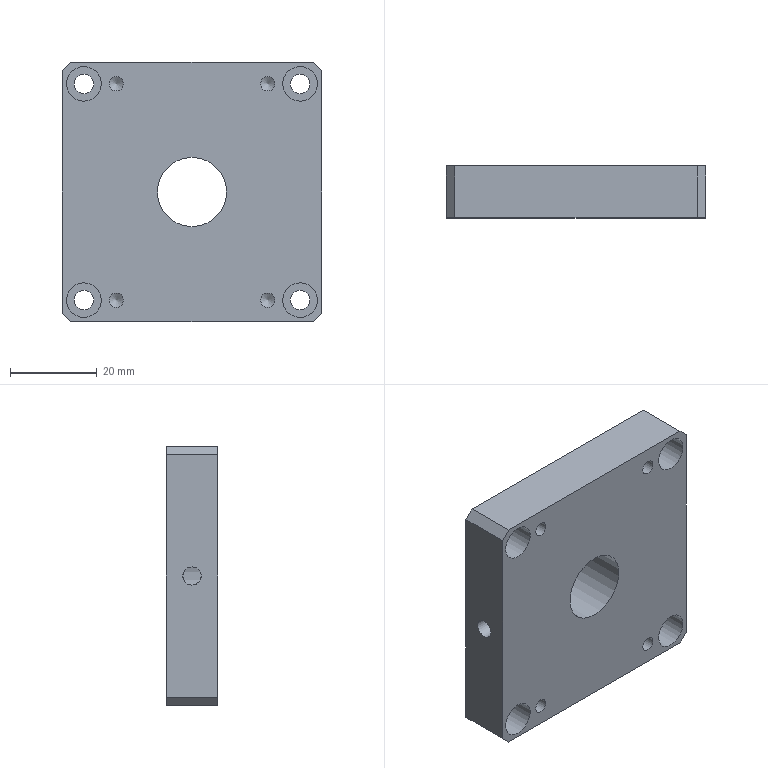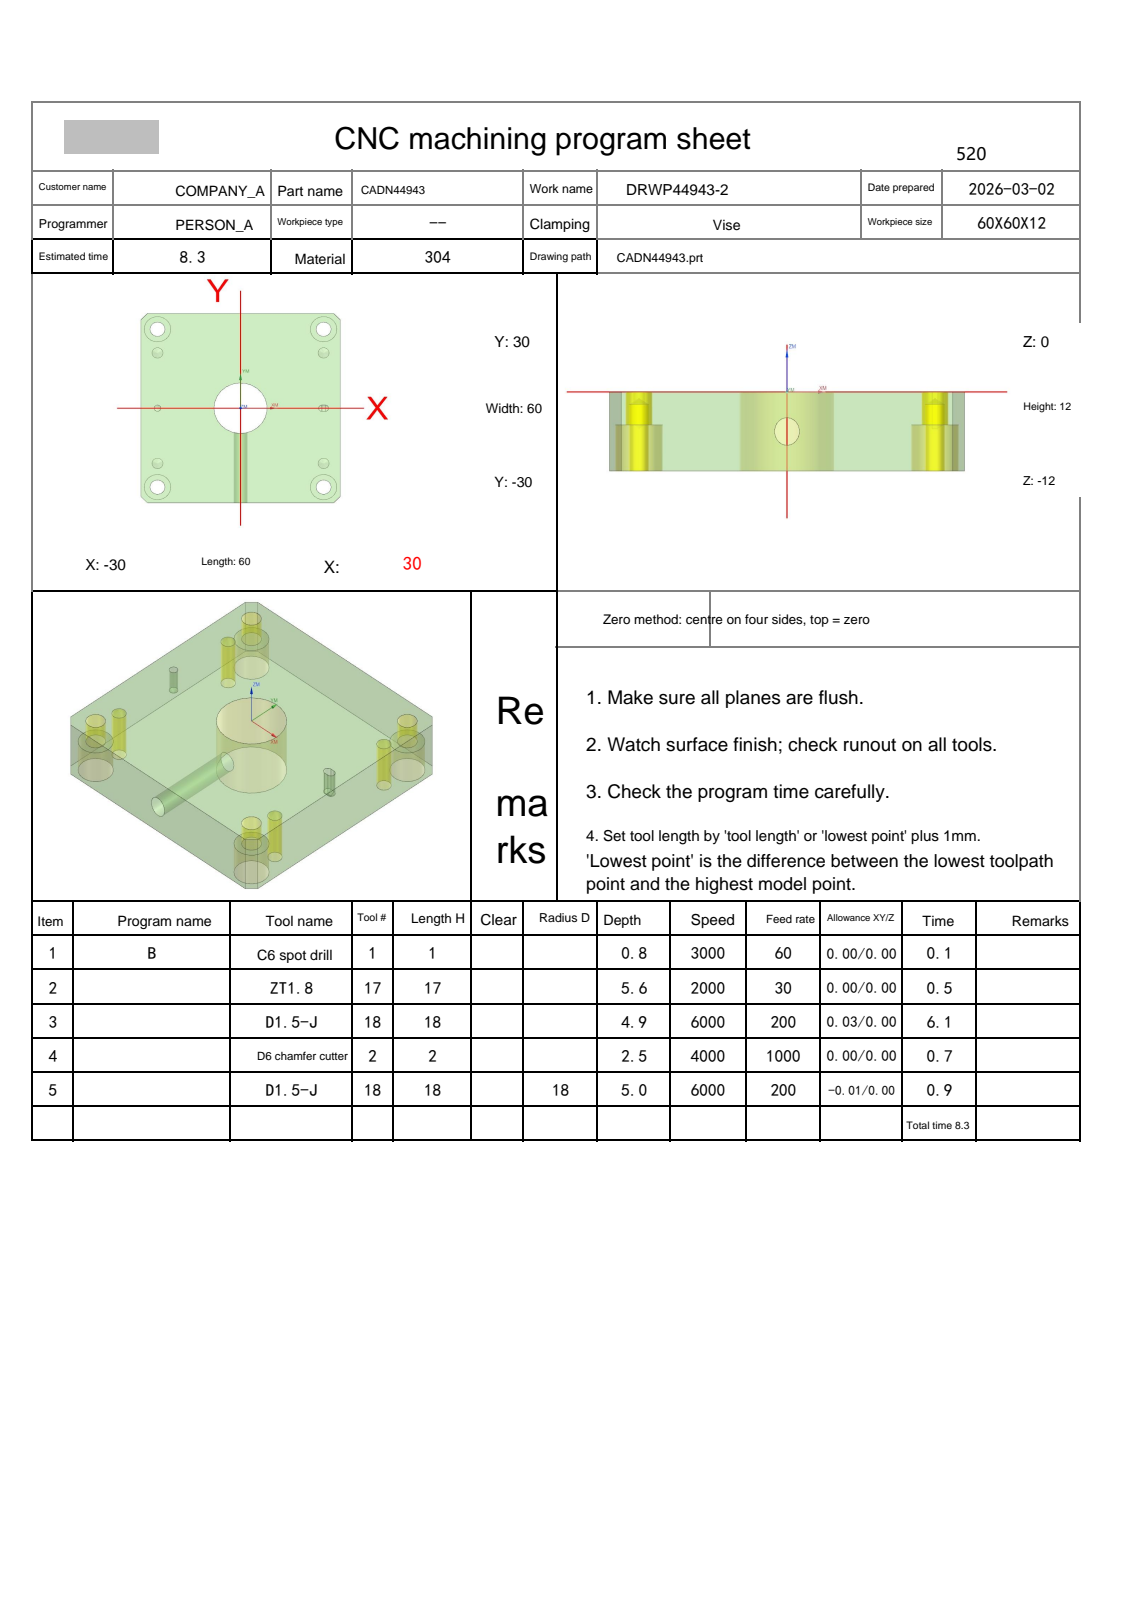NC program | NX | posted by the shop | part box 60 x 12 x 60 mm
Lines 42 to 868 of 3254:
N3 T18 M06
(D1.5-J  D=1.5 R=0. H=18 ce=0.03 di=0.00)
G00 G90 G54 X-25.22 Y.037 M03 S6000
G43 H18 Z50.
M08
Z.8
G01 Y-.119 Z.792 F200.
X-25.119 Y-.22 Z.784
X-24.881 Z.772
X-24.78 Y-.119 Z.764
Y.119 Z.752
X-24.881 Y.22 Z.744
X-25.119 Z.732
X-25.22 Y.119 Z.724
Y-.119 Z.712
X-25.119 Y-.22 Z.705
X-24.881 Z.692
X-24.78 Y-.119 Z.685
Y.119 Z.672
X-24.881 Y.22 Z.665
X-25.119 Z.652
X-25.22 Y.119 Z.645
Y-.119 Z.632
X-25.119 Y-.22 Z.625
X-24.881 Z.612
X-24.78 Y-.119 Z.605
Y.119 Z.592
X-24.881 Y.22 Z.585
X-25.119 Z.572
X-25.22 Y.119 Z.565
Y-.119 Z.552
X-25.119 Y-.22 Z.545
X-24.881 Z.532
X-24.78 Y-.119 Z.525
Y.119 Z.513
X-24.881 Y.22 Z.505
X-25.119 Z.493
X-25.22 Y.119 Z.485
Y-.119 Z.473
X-25.119 Y-.22 Z.465
X-24.881 Z.453
X-24.78 Y-.119 Z.445
Y.119 Z.433
X-24.881 Y.22 Z.425
X-25.119 Z.413
X-25.22 Y.119 Z.405
Y-.119 Z.393
X-25.119 Y-.22 Z.385
X-24.881 Z.373
X-24.78 Y-.119 Z.365
Y.119 Z.353
X-24.881 Y.22 Z.345
X-25.119 Z.333
X-25.22 Y.119 Z.325
Y-.119 Z.313
X-25.119 Y-.22 Z.305
X-24.881 Z.293
X-24.78 Y-.119 Z.286
Y.119 Z.273
X-24.881 Y.22 Z.266
X-25.119 Z.253
X-25.22 Y.119 Z.246
Y-.119 Z.233
X-25.119 Y-.22 Z.226
X-24.881 Z.213
X-24.78 Y-.119 Z.206
Y.119 Z.193
X-24.881 Y.22 Z.186
X-25.119 Z.173
X-25.22 Y.119 Z.166
Y-.119 Z.153
X-25.119 Y-.22 Z.146
X-24.881 Z.133
X-24.78 Y-.119 Z.126
Y.119 Z.113
X-24.881 Y.22 Z.106
X-25.119 Z.094
X-25.22 Y.119 Z.086
Y-.119 Z.074
X-25.119 Y-.22 Z.066
X-24.881 Z.054
X-24.78 Y-.119 Z.046
Y.119 Z.034
X-24.881 Y.22 Z.026
X-25.119 Z.014
X-25.22 Y.119 Z.006
Y0.0 Z0.0
G03 X-25. Y-.22 Z-.005 I.22 J0.0
X-24.78 Y0.0 Z-.01 I0.0 J.22
X-25. Y.22 Z-.015 I-.22 J0.0
X-25.22 Y0.0 Z-.02 I0.0 J-.22
X-25. Y-.22 Z-.025 I.22 J0.0
X-24.78 Y0.0 Z-.03 I0.0 J.22
X-25. Y.22 Z-.035 I-.22 J0.0
X-25.22 Y0.0 Z-.04 I0.0 J-.22
X-25. Y-.22 Z-.045 I.22 J0.0
X-24.78 Y0.0 Z-.05 I0.0 J.22
X-25. Y.22 Z-.055 I-.22 J0.0
X-25.22 Y0.0 Z-.06 I0.0 J-.22
X-25. Y-.22 Z-.065 I.22 J0.0
X-24.78 Y0.0 Z-.07 I0.0 J.22
X-25. Y.22 Z-.075 I-.22 J0.0
X-25.22 Y0.0 Z-.08 I0.0 J-.22
X-25. Y-.22 Z-.085 I.22 J0.0
X-24.78 Y0.0 Z-.09 I0.0 J.22
X-25. Y.22 Z-.095 I-.22 J0.0
X-25.22 Y0.0 Z-.1 I0.0 J-.22
X-25. Y-.22 Z-.105 I.22 J0.0
X-24.78 Y0.0 Z-.11 I0.0 J.22
X-25. Y.22 Z-.115 I-.22 J0.0
X-25.22 Y0.0 Z-.12 I0.0 J-.22
X-25. Y-.22 Z-.124 I.22 J0.0
X-24.78 Y0.0 Z-.129 I0.0 J.22
X-25. Y.22 Z-.134 I-.22 J0.0
X-25.22 Y0.0 Z-.139 I0.0 J-.22
X-25. Y-.22 Z-.144 I.22 J0.0
X-24.78 Y0.0 Z-.149 I0.0 J.22
X-25. Y.22 Z-.154 I-.22 J0.0
X-25.22 Y0.0 Z-.159 I0.0 J-.22
X-25. Y-.22 Z-.164 I.22 J0.0
X-24.78 Y0.0 Z-.169 I0.0 J.22
X-25. Y.22 Z-.174 I-.22 J0.0
X-25.22 Y0.0 Z-.179 I0.0 J-.22
X-25. Y-.22 Z-.184 I.22 J0.0
X-24.78 Y0.0 Z-.189 I0.0 J.22
X-25. Y.22 Z-.194 I-.22 J0.0
X-25.22 Y0.0 Z-.199 I0.0 J-.22
X-25. Y-.22 Z-.204 I.22 J0.0
X-24.78 Y0.0 Z-.209 I0.0 J.22
X-25. Y.22 Z-.214 I-.22 J0.0
X-25.22 Y0.0 Z-.219 I0.0 J-.22
X-25. Y-.22 Z-.224 I.22 J0.0
X-24.78 Y0.0 Z-.229 I0.0 J.22
X-25. Y.22 Z-.234 I-.22 J0.0
X-25.22 Y0.0 Z-.239 I0.0 J-.22
X-25. Y-.22 Z-.244 I.22 J0.0
X-24.78 Y0.0 Z-.249 I0.0 J.22
X-25. Y.22 Z-.254 I-.22 J0.0
X-25.22 Y0.0 Z-.259 I0.0 J-.22
X-25. Y-.22 Z-.264 I.22 J0.0
X-24.78 Y0.0 Z-.269 I0.0 J.22
X-25. Y.22 Z-.274 I-.22 J0.0
X-25.22 Y0.0 Z-.279 I0.0 J-.22
X-25. Y-.22 Z-.284 I.22 J0.0
X-24.78 Y0.0 Z-.289 I0.0 J.22
X-25. Y.22 Z-.294 I-.22 J0.0
X-25.22 Y0.0 Z-.299 I0.0 J-.22
X-25. Y-.22 Z-.304 I.22 J0.0
X-24.78 Y0.0 Z-.309 I0.0 J.22
X-25. Y.22 Z-.314 I-.22 J0.0
X-25.22 Y0.0 Z-.319 I0.0 J-.22
X-25. Y-.22 Z-.324 I.22 J0.0
X-24.78 Y0.0 Z-.329 I0.0 J.22
X-25. Y.22 Z-.334 I-.22 J0.0
X-25.22 Y0.0 Z-.339 I0.0 J-.22
X-25. Y-.22 Z-.344 I.22 J0.0
X-24.78 Y0.0 Z-.349 I0.0 J.22
X-25. Y.22 Z-.354 I-.22 J0.0
X-25.22 Y0.0 Z-.359 I0.0 J-.22
X-25. Y-.22 Z-.364 I.22 J0.0
X-24.78 Y0.0 Z-.369 I0.0 J.22
X-25. Y.22 Z-.373 I-.22 J0.0
X-25.22 Y0.0 Z-.378 I0.0 J-.22
X-25. Y-.22 Z-.383 I.22 J0.0
X-24.78 Y0.0 Z-.388 I0.0 J.22
X-25. Y.22 Z-.393 I-.22 J0.0
X-25.22 Y0.0 Z-.398 I0.0 J-.22
X-25. Y-.22 Z-.403 I.22 J0.0
X-24.78 Y0.0 Z-.408 I0.0 J.22
X-25. Y.22 Z-.413 I-.22 J0.0
X-25.22 Y0.0 Z-.418 I0.0 J-.22
X-25. Y-.22 Z-.423 I.22 J0.0
X-24.78 Y0.0 Z-.428 I0.0 J.22
X-25. Y.22 Z-.433 I-.22 J0.0
X-25.22 Y0.0 Z-.438 I0.0 J-.22
X-25. Y-.22 Z-.443 I.22 J0.0
X-24.78 Y0.0 Z-.448 I0.0 J.22
X-25. Y.22 Z-.453 I-.22 J0.0
X-25.22 Y0.0 Z-.458 I0.0 J-.22
X-25. Y-.22 Z-.463 I.22 J0.0
X-24.78 Y0.0 Z-.468 I0.0 J.22
X-25. Y.22 Z-.473 I-.22 J0.0
X-25.22 Y0.0 Z-.478 I0.0 J-.22
X-25. Y-.22 Z-.483 I.22 J0.0
X-24.78 Y0.0 Z-.488 I0.0 J.22
X-25. Y.22 Z-.493 I-.22 J0.0
X-25.22 Y0.0 Z-.498 I0.0 J-.22
X-25. Y-.22 Z-.503 I.22 J0.0
X-24.78 Y0.0 Z-.508 I0.0 J.22
X-25. Y.22 Z-.513 I-.22 J0.0
X-25.22 Y0.0 Z-.518 I0.0 J-.22
X-25. Y-.22 Z-.523 I.22 J0.0
X-24.78 Y0.0 Z-.528 I0.0 J.22
X-25. Y.22 Z-.533 I-.22 J0.0
X-25.22 Y0.0 Z-.538 I0.0 J-.22
X-25. Y-.22 Z-.543 I.22 J0.0
X-24.78 Y0.0 Z-.548 I0.0 J.22
X-25. Y.22 Z-.553 I-.22 J0.0
X-25.22 Y0.0 Z-.558 I0.0 J-.22
X-25. Y-.22 Z-.563 I.22 J0.0
X-24.78 Y0.0 Z-.568 I0.0 J.22
X-25. Y.22 Z-.573 I-.22 J0.0
X-25.22 Y0.0 Z-.578 I0.0 J-.22
X-25. Y-.22 Z-.583 I.22 J0.0
X-24.78 Y0.0 Z-.588 I0.0 J.22
X-25. Y.22 Z-.593 I-.22 J0.0
X-25.22 Y0.0 Z-.598 I0.0 J-.22
X-25. Y-.22 Z-.603 I.22 J0.0
X-24.78 Y0.0 Z-.608 I0.0 J.22
X-25. Y.22 Z-.613 I-.22 J0.0
X-25.22 Y0.0 Z-.618 I0.0 J-.22
X-25. Y-.22 Z-.622 I.22 J0.0
X-24.78 Y0.0 Z-.627 I0.0 J.22
X-25. Y.22 Z-.632 I-.22 J0.0
X-25.22 Y0.0 Z-.637 I0.0 J-.22
X-25. Y-.22 Z-.642 I.22 J0.0
X-24.78 Y0.0 Z-.647 I0.0 J.22
X-25. Y.22 Z-.652 I-.22 J0.0
X-25.22 Y0.0 Z-.657 I0.0 J-.22
X-25. Y-.22 Z-.662 I.22 J0.0
X-24.78 Y0.0 Z-.667 I0.0 J.22
X-25. Y.22 Z-.672 I-.22 J0.0
X-25.22 Y0.0 Z-.677 I0.0 J-.22
X-25. Y-.22 Z-.682 I.22 J0.0
X-24.78 Y0.0 Z-.687 I0.0 J.22
X-25. Y.22 Z-.692 I-.22 J0.0
X-25.22 Y0.0 Z-.697 I0.0 J-.22
X-25. Y-.22 Z-.702 I.22 J0.0
X-24.78 Y0.0 Z-.707 I0.0 J.22
X-25. Y.22 Z-.712 I-.22 J0.0
X-25.22 Y0.0 Z-.717 I0.0 J-.22
X-25. Y-.22 Z-.722 I.22 J0.0
X-24.78 Y0.0 Z-.727 I0.0 J.22
X-25. Y.22 Z-.732 I-.22 J0.0
X-25.22 Y0.0 Z-.737 I0.0 J-.22
X-25. Y-.22 Z-.742 I.22 J0.0
X-24.78 Y0.0 Z-.747 I0.0 J.22
X-25. Y.22 Z-.752 I-.22 J0.0
X-25.22 Y0.0 Z-.757 I0.0 J-.22
X-25. Y-.22 Z-.762 I.22 J0.0
X-24.78 Y0.0 Z-.767 I0.0 J.22
X-25. Y.22 Z-.772 I-.22 J0.0
X-25.22 Y0.0 Z-.777 I0.0 J-.22
X-25. Y-.22 Z-.782 I.22 J0.0
X-24.78 Y0.0 Z-.787 I0.0 J.22
X-25. Y.22 Z-.792 I-.22 J0.0
X-25.22 Y0.0 Z-.797 I0.0 J-.22
X-25. Y-.22 Z-.802 I.22 J0.0
X-24.78 Y0.0 Z-.807 I0.0 J.22
X-25. Y.22 Z-.812 I-.22 J0.0
X-25.22 Y0.0 Z-.817 I0.0 J-.22
X-25. Y-.22 Z-.822 I.22 J0.0
X-24.78 Y0.0 Z-.827 I0.0 J.22
X-25. Y.22 Z-.832 I-.22 J0.0
X-25.22 Y0.0 Z-.837 I0.0 J-.22
X-25. Y-.22 Z-.842 I.22 J0.0
X-24.78 Y0.0 Z-.847 I0.0 J.22
X-25. Y.22 Z-.852 I-.22 J0.0
X-25.22 Y0.0 Z-.857 I0.0 J-.22
X-25. Y-.22 Z-.862 I.22 J0.0
X-24.78 Y0.0 Z-.866 I0.0 J.22
X-25. Y.22 Z-.871 I-.22 J0.0
X-25.22 Y0.0 Z-.876 I0.0 J-.22
X-25. Y-.22 Z-.881 I.22 J0.0
X-24.78 Y0.0 Z-.886 I0.0 J.22
X-25. Y.22 Z-.891 I-.22 J0.0
X-25.22 Y0.0 Z-.896 I0.0 J-.22
X-25. Y-.22 Z-.901 I.22 J0.0
X-24.78 Y0.0 Z-.906 I0.0 J.22
X-25. Y.22 Z-.911 I-.22 J0.0
X-25.22 Y0.0 Z-.916 I0.0 J-.22
X-25. Y-.22 Z-.921 I.22 J0.0
X-24.78 Y0.0 Z-.926 I0.0 J.22
X-25. Y.22 Z-.931 I-.22 J0.0
X-25.22 Y0.0 Z-.936 I0.0 J-.22
X-25. Y-.22 Z-.941 I.22 J0.0
X-24.78 Y0.0 Z-.946 I0.0 J.22
X-25. Y.22 Z-.951 I-.22 J0.0
X-25.22 Y0.0 Z-.956 I0.0 J-.22
X-25. Y-.22 Z-.961 I.22 J0.0
X-24.78 Y0.0 Z-.966 I0.0 J.22
X-25. Y.22 Z-.971 I-.22 J0.0
X-25.22 Y0.0 Z-.976 I0.0 J-.22
X-25. Y-.22 Z-.981 I.22 J0.0
X-24.78 Y0.0 Z-.986 I0.0 J.22
X-25. Y.22 Z-.991 I-.22 J0.0
X-25.22 Y0.0 Z-.996 I0.0 J-.22
X-25. Y-.22 Z-1.001 I.22 J0.0
X-24.78 Y0.0 Z-1.006 I0.0 J.22
X-25. Y.22 Z-1.011 I-.22 J0.0
X-25.22 Y0.0 Z-1.016 I0.0 J-.22
X-25. Y-.22 Z-1.021 I.22 J0.0
X-24.78 Y0.0 Z-1.026 I0.0 J.22
X-25. Y.22 Z-1.031 I-.22 J0.0
X-25.22 Y0.0 Z-1.036 I0.0 J-.22
X-25. Y-.22 Z-1.041 I.22 J0.0
X-24.78 Y0.0 Z-1.046 I0.0 J.22
X-25. Y.22 Z-1.051 I-.22 J0.0
X-25.22 Y0.0 Z-1.056 I0.0 J-.22
X-25. Y-.22 Z-1.061 I.22 J0.0
X-24.78 Y0.0 Z-1.066 I0.0 J.22
X-25. Y.22 Z-1.071 I-.22 J0.0
X-25.22 Y0.0 Z-1.076 I0.0 J-.22
X-25. Y-.22 Z-1.081 I.22 J0.0
X-24.78 Y0.0 Z-1.086 I0.0 J.22
X-25. Y.22 Z-1.091 I-.22 J0.0
X-25.22 Y0.0 Z-1.096 I0.0 J-.22
X-25. Y-.22 Z-1.101 I.22 J0.0
X-24.78 Y0.0 Z-1.106 I0.0 J.22
X-25. Y.22 Z-1.111 I-.22 J0.0
X-25.22 Y0.0 Z-1.115 I0.0 J-.22
X-25. Y-.22 Z-1.12 I.22 J0.0
X-24.78 Y0.0 Z-1.125 I0.0 J.22
X-25. Y.22 Z-1.13 I-.22 J0.0
X-25.22 Y0.0 Z-1.135 I0.0 J-.22
X-25. Y-.22 Z-1.14 I.22 J0.0
X-24.78 Y0.0 Z-1.145 I0.0 J.22
X-25. Y.22 Z-1.15 I-.22 J0.0
X-25.22 Y0.0 Z-1.155 I0.0 J-.22
X-25. Y-.22 Z-1.16 I.22 J0.0
X-24.78 Y0.0 Z-1.165 I0.0 J.22
X-25. Y.22 Z-1.17 I-.22 J0.0
X-25.22 Y0.0 Z-1.175 I0.0 J-.22
X-25. Y-.22 Z-1.18 I.22 J0.0
X-24.78 Y0.0 Z-1.185 I0.0 J.22
X-25. Y.22 Z-1.19 I-.22 J0.0
X-25.22 Y0.0 Z-1.195 I0.0 J-.22
X-25. Y-.22 Z-1.2 I.22 J0.0
X-24.78 Y0.0 Z-1.205 I0.0 J.22
X-25. Y.22 Z-1.21 I-.22 J0.0
X-25.22 Y0.0 Z-1.215 I0.0 J-.22
X-25. Y-.22 Z-1.22 I.22 J0.0
X-24.78 Y0.0 Z-1.225 I0.0 J.22
X-25. Y.22 Z-1.23 I-.22 J0.0
X-25.22 Y0.0 Z-1.235 I0.0 J-.22
X-25. Y-.22 Z-1.24 I.22 J0.0
X-24.78 Y0.0 Z-1.245 I0.0 J.22
X-25. Y.22 Z-1.25 I-.22 J0.0
X-25.22 Y0.0 Z-1.255 I0.0 J-.22
X-25. Y-.22 Z-1.26 I.22 J0.0
X-24.78 Y0.0 Z-1.265 I0.0 J.22
X-25. Y.22 Z-1.27 I-.22 J0.0
X-25.22 Y0.0 Z-1.275 I0.0 J-.22
X-25. Y-.22 Z-1.28 I.22 J0.0
X-24.78 Y0.0 Z-1.285 I0.0 J.22
X-25. Y.22 Z-1.29 I-.22 J0.0
X-25.22 Y0.0 Z-1.295 I0.0 J-.22
X-25. Y-.22 Z-1.3 I.22 J0.0
X-24.78 Y0.0 Z-1.305 I0.0 J.22
X-25. Y.22 Z-1.31 I-.22 J0.0
X-25.22 Y0.0 Z-1.315 I0.0 J-.22
X-25. Y-.22 Z-1.32 I.22 J0.0
X-24.78 Y0.0 Z-1.325 I0.0 J.22
X-25. Y.22 Z-1.33 I-.22 J0.0
X-25.22 Y0.0 Z-1.335 I0.0 J-.22
X-25. Y-.22 Z-1.34 I.22 J0.0
X-24.78 Y0.0 Z-1.345 I0.0 J.22
X-25. Y.22 Z-1.35 I-.22 J0.0
X-25.22 Y0.0 Z-1.355 I0.0 J-.22
X-25. Y-.22 Z-1.359 I.22 J0.0
X-24.78 Y0.0 Z-1.364 I0.0 J.22
X-25. Y.22 Z-1.369 I-.22 J0.0
X-25.22 Y0.0 Z-1.374 I0.0 J-.22
X-25. Y-.22 Z-1.379 I.22 J0.0
X-24.78 Y0.0 Z-1.384 I0.0 J.22
X-25. Y.22 Z-1.389 I-.22 J0.0
X-25.22 Y0.0 Z-1.394 I0.0 J-.22
X-25. Y-.22 Z-1.399 I.22 J0.0
X-24.78 Y0.0 Z-1.404 I0.0 J.22
X-25. Y.22 Z-1.409 I-.22 J0.0
X-25.22 Y0.0 Z-1.414 I0.0 J-.22
X-25. Y-.22 Z-1.419 I.22 J0.0
X-24.78 Y0.0 Z-1.424 I0.0 J.22
X-25. Y.22 Z-1.429 I-.22 J0.0
X-25.22 Y0.0 Z-1.434 I0.0 J-.22
X-25. Y-.22 Z-1.439 I.22 J0.0
X-24.78 Y0.0 Z-1.444 I0.0 J.22
X-25. Y.22 Z-1.449 I-.22 J0.0
X-25.22 Y0.0 Z-1.454 I0.0 J-.22
X-25. Y-.22 Z-1.459 I.22 J0.0
X-24.78 Y0.0 Z-1.464 I0.0 J.22
X-25. Y.22 Z-1.469 I-.22 J0.0
X-25.22 Y0.0 Z-1.474 I0.0 J-.22
X-25. Y-.22 Z-1.479 I.22 J0.0
X-24.78 Y0.0 Z-1.484 I0.0 J.22
X-25. Y.22 Z-1.489 I-.22 J0.0
X-25.22 Y0.0 Z-1.494 I0.0 J-.22
X-25. Y-.22 Z-1.499 I.22 J0.0
X-24.78 Y0.0 Z-1.504 I0.0 J.22
X-25. Y.22 Z-1.509 I-.22 J0.0
X-25.22 Y0.0 Z-1.514 I0.0 J-.22
X-25. Y-.22 Z-1.519 I.22 J0.0
X-24.78 Y0.0 Z-1.524 I0.0 J.22
X-25. Y.22 Z-1.529 I-.22 J0.0
X-25.22 Y0.0 Z-1.534 I0.0 J-.22
X-25. Y-.22 Z-1.539 I.22 J0.0
X-24.78 Y0.0 Z-1.544 I0.0 J.22
X-25. Y.22 Z-1.549 I-.22 J0.0
X-25.22 Y0.0 Z-1.554 I0.0 J-.22
X-25. Y-.22 Z-1.559 I.22 J0.0
X-24.78 Y0.0 Z-1.564 I0.0 J.22
X-25. Y.22 Z-1.569 I-.22 J0.0
X-25.22 Y0.0 Z-1.574 I0.0 J-.22
X-25. Y-.22 Z-1.579 I.22 J0.0
X-24.78 Y0.0 Z-1.584 I0.0 J.22
X-25. Y.22 Z-1.589 I-.22 J0.0
X-25.22 Y0.0 Z-1.594 I0.0 J-.22
X-25. Y-.22 Z-1.599 I.22 J0.0
X-24.78 Y0.0 Z-1.604 I0.0 J.22
X-25. Y.22 Z-1.608 I-.22 J0.0
X-25.22 Y0.0 Z-1.613 I0.0 J-.22
X-25. Y-.22 Z-1.618 I.22 J0.0
X-24.78 Y0.0 Z-1.623 I0.0 J.22
X-25. Y.22 Z-1.628 I-.22 J0.0
X-25.22 Y0.0 Z-1.633 I0.0 J-.22
X-25. Y-.22 Z-1.638 I.22 J0.0
X-24.78 Y0.0 Z-1.643 I0.0 J.22
X-25. Y.22 Z-1.648 I-.22 J0.0
X-25.22 Y0.0 Z-1.653 I0.0 J-.22
X-25. Y-.22 Z-1.658 I.22 J0.0
X-24.78 Y0.0 Z-1.663 I0.0 J.22
X-25. Y.22 Z-1.668 I-.22 J0.0
X-25.22 Y0.0 Z-1.673 I0.0 J-.22
X-25. Y-.22 Z-1.678 I.22 J0.0
X-24.78 Y0.0 Z-1.683 I0.0 J.22
X-25. Y.22 Z-1.688 I-.22 J0.0
X-25.22 Y0.0 Z-1.693 I0.0 J-.22
X-25. Y-.22 Z-1.698 I.22 J0.0
X-24.78 Y0.0 Z-1.703 I0.0 J.22
X-25. Y.22 Z-1.708 I-.22 J0.0
X-25.22 Y0.0 Z-1.713 I0.0 J-.22
X-25. Y-.22 Z-1.718 I.22 J0.0
X-24.78 Y0.0 Z-1.723 I0.0 J.22
X-25. Y.22 Z-1.728 I-.22 J0.0
X-25.22 Y0.0 Z-1.733 I0.0 J-.22
X-25. Y-.22 Z-1.738 I.22 J0.0
X-24.78 Y0.0 Z-1.743 I0.0 J.22
X-25. Y.22 Z-1.748 I-.22 J0.0
X-25.22 Y0.0 Z-1.753 I0.0 J-.22
X-25. Y-.22 Z-1.758 I.22 J0.0
X-24.78 Y0.0 Z-1.763 I0.0 J.22
X-25. Y.22 Z-1.768 I-.22 J0.0
X-25.22 Y0.0 Z-1.773 I0.0 J-.22
X-25. Y-.22 Z-1.778 I.22 J0.0
X-24.78 Y0.0 Z-1.783 I0.0 J.22
X-25. Y.22 Z-1.788 I-.22 J0.0
X-25.22 Y0.0 Z-1.793 I0.0 J-.22
X-25. Y-.22 Z-1.798 I.22 J0.0
X-24.78 Y0.0 Z-1.803 I0.0 J.22
X-25. Y.22 Z-1.808 I-.22 J0.0
X-25.22 Y0.0 Z-1.813 I0.0 J-.22
X-25. Y-.22 Z-1.818 I.22 J0.0
X-24.78 Y0.0 Z-1.823 I0.0 J.22
X-25. Y.22 Z-1.828 I-.22 J0.0
X-25.22 Y0.0 Z-1.833 I0.0 J-.22
X-25. Y-.22 Z-1.838 I.22 J0.0
X-24.78 Y0.0 Z-1.843 I0.0 J.22
X-25. Y.22 Z-1.848 I-.22 J0.0
X-25.22 Y0.0 Z-1.853 I0.0 J-.22
X-25. Y-.22 Z-1.857 I.22 J0.0
X-24.78 Y0.0 Z-1.862 I0.0 J.22
X-25. Y.22 Z-1.867 I-.22 J0.0
X-25.22 Y0.0 Z-1.872 I0.0 J-.22
X-25. Y-.22 Z-1.877 I.22 J0.0
X-24.78 Y0.0 Z-1.882 I0.0 J.22
X-25. Y.22 Z-1.887 I-.22 J0.0
X-25.22 Y0.0 Z-1.892 I0.0 J-.22
X-25. Y-.22 Z-1.897 I.22 J0.0
X-24.78 Y0.0 Z-1.902 I0.0 J.22
X-25. Y.22 Z-1.907 I-.22 J0.0
X-25.22 Y0.0 Z-1.912 I0.0 J-.22
X-25. Y-.22 Z-1.917 I.22 J0.0
X-24.78 Y0.0 Z-1.922 I0.0 J.22
X-25. Y.22 Z-1.927 I-.22 J0.0
X-25.22 Y0.0 Z-1.932 I0.0 J-.22
X-25. Y-.22 Z-1.937 I.22 J0.0
X-24.78 Y0.0 Z-1.942 I0.0 J.22
X-25. Y.22 Z-1.947 I-.22 J0.0
X-25.22 Y0.0 Z-1.952 I0.0 J-.22
X-25. Y-.22 Z-1.957 I.22 J0.0
X-24.78 Y0.0 Z-1.962 I0.0 J.22
X-25. Y.22 Z-1.967 I-.22 J0.0
X-25.22 Y0.0 Z-1.972 I0.0 J-.22
X-25. Y-.22 Z-1.977 I.22 J0.0
X-24.78 Y0.0 Z-1.982 I0.0 J.22
X-25. Y.22 Z-1.987 I-.22 J0.0
X-25.22 Y0.0 Z-1.992 I0.0 J-.22
X-25. Y-.22 Z-1.997 I.22 J0.0
X-24.78 Y0.0 Z-2.002 I0.0 J.22
X-25. Y.22 Z-2.007 I-.22 J0.0
X-25.22 Y0.0 Z-2.012 I0.0 J-.22
X-25. Y-.22 Z-2.017 I.22 J0.0
X-24.78 Y0.0 Z-2.022 I0.0 J.22
X-25. Y.22 Z-2.027 I-.22 J0.0
X-25.22 Y0.0 Z-2.032 I0.0 J-.22
X-25. Y-.22 Z-2.037 I.22 J0.0
X-24.78 Y0.0 Z-2.042 I0.0 J.22
X-25. Y.22 Z-2.047 I-.22 J0.0
X-25.22 Y0.0 Z-2.052 I0.0 J-.22
X-25. Y-.22 Z-2.057 I.22 J0.0
X-24.78 Y0.0 Z-2.062 I0.0 J.22
X-25. Y.22 Z-2.067 I-.22 J0.0
X-25.22 Y0.0 Z-2.072 I0.0 J-.22
X-25. Y-.22 Z-2.077 I.22 J0.0
X-24.78 Y0.0 Z-2.082 I0.0 J.22
X-25. Y.22 Z-2.087 I-.22 J0.0
X-25.22 Y0.0 Z-2.092 I0.0 J-.22
X-25. Y-.22 Z-2.097 I.22 J0.0
X-24.78 Y0.0 Z-2.101 I0.0 J.22
X-25. Y.22 Z-2.106 I-.22 J0.0
X-25.22 Y0.0 Z-2.111 I0.0 J-.22
X-25. Y-.22 Z-2.116 I.22 J0.0
X-24.78 Y0.0 Z-2.121 I0.0 J.22
X-25. Y.22 Z-2.126 I-.22 J0.0
X-25.22 Y0.0 Z-2.131 I0.0 J-.22
X-25. Y-.22 Z-2.136 I.22 J0.0
X-24.78 Y0.0 Z-2.141 I0.0 J.22
X-25. Y.22 Z-2.146 I-.22 J0.0
X-25.22 Y0.0 Z-2.151 I0.0 J-.22
X-25. Y-.22 Z-2.156 I.22 J0.0
X-24.78 Y0.0 Z-2.161 I0.0 J.22
X-25. Y.22 Z-2.166 I-.22 J0.0
X-25.22 Y0.0 Z-2.171 I0.0 J-.22
X-25. Y-.22 Z-2.176 I.22 J0.0
X-24.78 Y0.0 Z-2.181 I0.0 J.22
X-25. Y.22 Z-2.186 I-.22 J0.0
X-25.22 Y0.0 Z-2.191 I0.0 J-.22
X-25. Y-.22 Z-2.196 I.22 J0.0
X-24.78 Y0.0 Z-2.201 I0.0 J.22
X-25. Y.22 Z-2.206 I-.22 J0.0
X-25.22 Y0.0 Z-2.211 I0.0 J-.22
X-25. Y-.22 Z-2.216 I.22 J0.0
X-24.78 Y0.0 Z-2.221 I0.0 J.22
X-25. Y.22 Z-2.226 I-.22 J0.0
X-25.22 Y0.0 Z-2.231 I0.0 J-.22
X-25. Y-.22 Z-2.236 I.22 J0.0
X-24.78 Y0.0 Z-2.241 I0.0 J.22
X-25. Y.22 Z-2.246 I-.22 J0.0
X-25.22 Y0.0 Z-2.251 I0.0 J-.22
X-25. Y-.22 Z-2.256 I.22 J0.0
X-24.78 Y0.0 Z-2.261 I0.0 J.22
X-25. Y.22 Z-2.266 I-.22 J0.0
X-25.22 Y0.0 Z-2.271 I0.0 J-.22
X-25. Y-.22 Z-2.276 I.22 J0.0
X-24.78 Y0.0 Z-2.281 I0.0 J.22
X-25. Y.22 Z-2.286 I-.22 J0.0
X-25.22 Y0.0 Z-2.291 I0.0 J-.22
X-25. Y-.22 Z-2.296 I.22 J0.0
X-24.78 Y0.0 Z-2.301 I0.0 J.22
X-25. Y.22 Z-2.306 I-.22 J0.0
X-25.22 Y0.0 Z-2.311 I0.0 J-.22
X-25. Y-.22 Z-2.316 I.22 J0.0
X-24.78 Y0.0 Z-2.321 I0.0 J.22
X-25. Y.22 Z-2.326 I-.22 J0.0
X-25.22 Y0.0 Z-2.331 I0.0 J-.22
X-25. Y-.22 Z-2.336 I.22 J0.0
X-24.78 Y0.0 Z-2.341 I0.0 J.22
X-25. Y.22 Z-2.346 I-.22 J0.0
X-25.22 Y0.0 Z-2.35 I0.0 J-.22
X-25. Y-.22 Z-2.355 I.22 J0.0
X-24.78 Y0.0 Z-2.36 I0.0 J.22
X-25. Y.22 Z-2.365 I-.22 J0.0
X-25.22 Y0.0 Z-2.37 I0.0 J-.22
X-25. Y-.22 Z-2.375 I.22 J0.0
X-24.78 Y0.0 Z-2.38 I0.0 J.22
X-25. Y.22 Z-2.385 I-.22 J0.0
X-25.22 Y0.0 Z-2.39 I0.0 J-.22
X-25. Y-.22 Z-2.395 I.22 J0.0
X-24.78 Y0.0 Z-2.4 I0.0 J.22
X-25. Y.22 Z-2.405 I-.22 J0.0
X-25.22 Y0.0 Z-2.41 I0.0 J-.22
X-25. Y-.22 Z-2.415 I.22 J0.0
X-24.78 Y0.0 Z-2.42 I0.0 J.22
X-25. Y.22 Z-2.425 I-.22 J0.0
X-25.22 Y0.0 Z-2.43 I0.0 J-.22
X-25. Y-.22 Z-2.435 I.22 J0.0
X-24.78 Y0.0 Z-2.44 I0.0 J.22
X-25. Y.22 Z-2.445 I-.22 J0.0
X-25.22 Y0.0 Z-2.45 I0.0 J-.22
X-25. Y-.22 Z-2.455 I.22 J0.0
X-24.78 Y0.0 Z-2.46 I0.0 J.22
X-25. Y.22 Z-2.465 I-.22 J0.0
X-25.22 Y0.0 Z-2.47 I0.0 J-.22
X-25. Y-.22 Z-2.475 I.22 J0.0
X-24.78 Y0.0 Z-2.48 I0.0 J.22
X-25. Y.22 Z-2.485 I-.22 J0.0
X-25.22 Y0.0 Z-2.49 I0.0 J-.22
X-25. Y-.22 Z-2.495 I.22 J0.0
X-24.78 Y0.0 Z-2.5 I0.0 J.22
X-25. Y.22 Z-2.505 I-.22 J0.0
X-25.22 Y0.0 Z-2.51 I0.0 J-.22
X-25. Y-.22 Z-2.515 I.22 J0.0
X-24.78 Y0.0 Z-2.52 I0.0 J.22
X-25. Y.22 Z-2.525 I-.22 J0.0
X-25.22 Y0.0 Z-2.53 I0.0 J-.22
X-25. Y-.22 Z-2.535 I.22 J0.0
X-24.78 Y0.0 Z-2.54 I0.0 J.22
X-25. Y.22 Z-2.545 I-.22 J0.0
X-25.22 Y0.0 Z-2.55 I0.0 J-.22
X-25. Y-.22 Z-2.555 I.22 J0.0
X-24.78 Y0.0 Z-2.56 I0.0 J.22
X-25. Y.22 Z-2.565 I-.22 J0.0
X-25.22 Y0.0 Z-2.57 I0.0 J-.22
X-25. Y-.22 Z-2.575 I.22 J0.0
X-24.78 Y0.0 Z-2.58 I0.0 J.22
X-25. Y.22 Z-2.585 I-.22 J0.0
X-25.22 Y0.0 Z-2.59 I0.0 J-.22
X-25. Y-.22 Z-2.594 I.22 J0.0
X-24.78 Y0.0 Z-2.599 I0.0 J.22
X-25. Y.22 Z-2.604 I-.22 J0.0
X-25.22 Y0.0 Z-2.609 I0.0 J-.22
X-25. Y-.22 Z-2.614 I.22 J0.0
X-24.78 Y0.0 Z-2.619 I0.0 J.22
X-25. Y.22 Z-2.624 I-.22 J0.0
X-25.22 Y0.0 Z-2.629 I0.0 J-.22
X-25. Y-.22 Z-2.634 I.22 J0.0
X-24.78 Y0.0 Z-2.639 I0.0 J.22
X-25. Y.22 Z-2.644 I-.22 J0.0
X-25.22 Y0.0 Z-2.649 I0.0 J-.22
X-25. Y-.22 Z-2.654 I.22 J0.0
X-24.78 Y0.0 Z-2.659 I0.0 J.22
X-25. Y.22 Z-2.664 I-.22 J0.0
X-25.22 Y0.0 Z-2.669 I0.0 J-.22
X-25. Y-.22 Z-2.674 I.22 J0.0
X-24.78 Y0.0 Z-2.679 I0.0 J.22
X-25. Y.22 Z-2.684 I-.22 J0.0
X-25.22 Y0.0 Z-2.689 I0.0 J-.22
X-25. Y-.22 Z-2.694 I.22 J0.0
X-24.78 Y0.0 Z-2.699 I0.0 J.22
X-25. Y.22 Z-2.704 I-.22 J0.0
X-25.22 Y0.0 Z-2.709 I0.0 J-.22
X-25. Y-.22 Z-2.714 I.22 J0.0
X-24.78 Y0.0 Z-2.719 I0.0 J.22
X-25. Y.22 Z-2.724 I-.22 J0.0
X-25.22 Y0.0 Z-2.729 I0.0 J-.22
X-25. Y-.22 Z-2.734 I.22 J0.0
X-24.78 Y0.0 Z-2.739 I0.0 J.22
X-25. Y.22 Z-2.744 I-.22 J0.0
X-25.22 Y0.0 Z-2.749 I0.0 J-.22
X-25. Y-.22 Z-2.754 I.22 J0.0
X-24.78 Y0.0 Z-2.759 I0.0 J.22
X-25. Y.22 Z-2.764 I-.22 J0.0
X-25.22 Y0.0 Z-2.769 I0.0 J-.22
X-25. Y-.22 Z-2.774 I.22 J0.0
X-24.78 Y0.0 Z-2.779 I0.0 J.22
X-25. Y.22 Z-2.784 I-.22 J0.0
X-25.22 Y0.0 Z-2.789 I0.0 J-.22
X-25. Y-.22 Z-2.794 I.22 J0.0
X-24.78 Y0.0 Z-2.799 I0.0 J.22
X-25. Y.22 Z-2.804 I-.22 J0.0
X-25.22 Y0.0 Z-2.809 I0.0 J-.22
X-25. Y-.22 Z-2.814 I.22 J0.0
X-24.78 Y0.0 Z-2.819 I0.0 J.22
X-25. Y.22 Z-2.824 I-.22 J0.0
X-25.22 Y0.0 Z-2.829 I0.0 J-.22
X-25. Y-.22 Z-2.834 I.22 J0.0
X-24.78 Y0.0 Z-2.839 I0.0 J.22
X-25. Y.22 Z-2.843 I-.22 J0.0
X-25.22 Y0.0 Z-2.848 I0.0 J-.22
X-25. Y-.22 Z-2.853 I.22 J0.0
X-24.78 Y0.0 Z-2.858 I0.0 J.22
X-25. Y.22 Z-2.863 I-.22 J0.0
X-25.22 Y0.0 Z-2.868 I0.0 J-.22
X-25. Y-.22 Z-2.873 I.22 J0.0
X-24.78 Y0.0 Z-2.878 I0.0 J.22
X-25. Y.22 Z-2.883 I-.22 J0.0
X-25.22 Y0.0 Z-2.888 I0.0 J-.22
X-25. Y-.22 Z-2.893 I.22 J0.0
X-24.78 Y0.0 Z-2.898 I0.0 J.22
X-25. Y.22 Z-2.903 I-.22 J0.0
X-25.22 Y0.0 Z-2.908 I0.0 J-.22
X-25. Y-.22 Z-2.913 I.22 J0.0
X-24.78 Y0.0 Z-2.918 I0.0 J.22
X-25. Y.22 Z-2.923 I-.22 J0.0
X-25.22 Y0.0 Z-2.928 I0.0 J-.22
X-25. Y-.22 Z-2.933 I.22 J0.0
X-24.78 Y0.0 Z-2.938 I0.0 J.22
X-25. Y.22 Z-2.943 I-.22 J0.0
X-25.22 Y0.0 Z-2.948 I0.0 J-.22
X-25. Y-.22 Z-2.953 I.22 J0.0
X-24.78 Y0.0 Z-2.958 I0.0 J.22
X-25. Y.22 Z-2.963 I-.22 J0.0
X-25.22 Y0.0 Z-2.968 I0.0 J-.22
X-25. Y-.22 Z-2.973 I.22 J0.0
X-24.78 Y0.0 Z-2.978 I0.0 J.22
X-25. Y.22 Z-2.983 I-.22 J0.0
X-25.22 Y0.0 Z-2.988 I0.0 J-.22
X-25. Y-.22 Z-2.993 I.22 J0.0
X-24.78 Y0.0 Z-2.998 I0.0 J.22
X-25. Y.22 Z-3.003 I-.22 J0.0
X-25.22 Y0.0 Z-3.008 I0.0 J-.22
X-25. Y-.22 Z-3.013 I.22 J0.0
X-24.78 Y0.0 Z-3.018 I0.0 J.22
X-25. Y.22 Z-3.023 I-.22 J0.0
X-25.22 Y0.0 Z-3.028 I0.0 J-.22
X-25. Y-.22 Z-3.033 I.22 J0.0
X-24.78 Y0.0 Z-3.038 I0.0 J.22
X-25. Y.22 Z-3.043 I-.22 J0.0
X-25.22 Y0.0 Z-3.048 I0.0 J-.22
X-25. Y-.22 Z-3.053 I.22 J0.0
X-24.78 Y0.0 Z-3.058 I0.0 J.22
X-25. Y.22 Z-3.063 I-.22 J0.0
X-25.22 Y0.0 Z-3.068 I0.0 J-.22
X-25. Y-.22 Z-3.073 I.22 J0.0
X-24.78 Y0.0 Z-3.078 I0.0 J.22
X-25. Y.22 Z-3.083 I-.22 J0.0
X-25.22 Y0.0 Z-3.088 I0.0 J-.22
X-25. Y-.22 Z-3.092 I.22 J0.0
X-24.78 Y0.0 Z-3.097 I0.0 J.22
X-25. Y.22 Z-3.102 I-.22 J0.0
X-25.22 Y0.0 Z-3.107 I0.0 J-.22
X-25. Y-.22 Z-3.112 I.22 J0.0
X-24.78 Y0.0 Z-3.117 I0.0 J.22
X-25. Y.22 Z-3.122 I-.22 J0.0
X-25.22 Y0.0 Z-3.127 I0.0 J-.22
X-25. Y-.22 Z-3.132 I.22 J0.0
X-24.78 Y0.0 Z-3.137 I0.0 J.22
X-25. Y.22 Z-3.142 I-.22 J0.0
X-25.22 Y0.0 Z-3.147 I0.0 J-.22
X-25. Y-.22 Z-3.152 I.22 J0.0
X-24.78 Y0.0 Z-3.157 I0.0 J.22
X-25. Y.22 Z-3.162 I-.22 J0.0
X-25.22 Y0.0 Z-3.167 I0.0 J-.22
X-25. Y-.22 Z-3.172 I.22 J0.0
X-24.78 Y0.0 Z-3.177 I0.0 J.22
X-25. Y.22 Z-3.182 I-.22 J0.0
X-25.22 Y0.0 Z-3.187 I0.0 J-.22
X-25. Y-.22 Z-3.192 I.22 J0.0
X-24.78 Y0.0 Z-3.197 I0.0 J.22
X-25. Y.22 Z-3.202 I-.22 J0.0
X-25.22 Y0.0 Z-3.207 I0.0 J-.22
X-25. Y-.22 Z-3.212 I.22 J0.0
X-24.78 Y0.0 Z-3.217 I0.0 J.22
X-25. Y.22 Z-3.222 I-.22 J0.0
X-25.22 Y0.0 Z-3.227 I0.0 J-.22
X-25. Y-.22 Z-3.232 I.22 J0.0
X-24.78 Y0.0 Z-3.237 I0.0 J.22
X-25. Y.22 Z-3.242 I-.22 J0.0
X-25.22 Y0.0 Z-3.247 I0.0 J-.22
X-25. Y-.22 Z-3.252 I.22 J0.0
X-24.78 Y0.0 Z-3.257 I0.0 J.22
X-25. Y.22 Z-3.262 I-.22 J0.0
X-25.22 Y0.0 Z-3.267 I0.0 J-.22
X-25. Y-.22 Z-3.272 I.22 J0.0
X-24.78 Y0.0 Z-3.277 I0.0 J.22
X-25. Y.22 Z-3.282 I-.22 J0.0
X-25.22 Y0.0 Z-3.287 I0.0 J-.22
X-25. Y-.22 Z-3.292 I.22 J0.0
X-24.78 Y0.0 Z-3.297 I0.0 J.22
X-25. Y.22 Z-3.302 I-.22 J0.0
X-25.22 Y0.0 Z-3.307 I0.0 J-.22
X-25. Y-.22 Z-3.312 I.22 J0.0
X-24.78 Y0.0 Z-3.317 I0.0 J.22
X-25. Y.22 Z-3.322 I-.22 J0.0
X-25.22 Y0.0 Z-3.327 I0.0 J-.22
X-25. Y-.22 Z-3.332 I.22 J0.0
X-24.78 Y0.0 Z-3.336 I0.0 J.22
X-25. Y.22 Z-3.341 I-.22 J0.0
X-25.22 Y0.0 Z-3.346 I0.0 J-.22
X-25. Y-.22 Z-3.351 I.22 J0.0
X-24.78 Y0.0 Z-3.356 I0.0 J.22
X-25. Y.22 Z-3.361 I-.22 J0.0
X-25.22 Y0.0 Z-3.366 I0.0 J-.22
X-25. Y-.22 Z-3.371 I.22 J0.0
X-24.78 Y0.0 Z-3.376 I0.0 J.22
X-25. Y.22 Z-3.381 I-.22 J0.0
X-25.22 Y0.0 Z-3.386 I0.0 J-.22
X-25. Y-.22 Z-3.391 I.22 J0.0
X-24.78 Y0.0 Z-3.396 I0.0 J.22
X-25. Y.22 Z-3.401 I-.22 J0.0
X-25.22 Y0.0 Z-3.406 I0.0 J-.22
X-25. Y-.22 Z-3.411 I.22 J0.0
X-24.78 Y0.0 Z-3.416 I0.0 J.22
X-25. Y.22 Z-3.421 I-.22 J0.0
X-25.22 Y0.0 Z-3.426 I0.0 J-.22
X-25. Y-.22 Z-3.431 I.22 J0.0
X-24.78 Y0.0 Z-3.436 I0.0 J.22
X-25. Y.22 Z-3.441 I-.22 J0.0
X-25.22 Y0.0 Z-3.446 I0.0 J-.22
X-25. Y-.22 Z-3.451 I.22 J0.0
X-24.78 Y0.0 Z-3.456 I0.0 J.22
X-25. Y.22 Z-3.461 I-.22 J0.0
X-25.22 Y0.0 Z-3.466 I0.0 J-.22
X-25. Y-.22 Z-3.471 I.22 J0.0
X-24.78 Y0.0 Z-3.476 I0.0 J.22
X-25. Y.22 Z-3.481 I-.22 J0.0
X-25.22 Y0.0 Z-3.486 I0.0 J-.22
X-25. Y-.22 Z-3.491 I.22 J0.0
X-24.78 Y0.0 Z-3.496 I0.0 J.22
X-25. Y.22 Z-3.501 I-.22 J0.0
X-25.22 Y0.0 Z-3.506 I0.0 J-.22
X-25. Y-.22 Z-3.511 I.22 J0.0
X-24.78 Y0.0 Z-3.516 I0.0 J.22
X-25. Y.22 Z-3.521 I-.22 J0.0
X-25.22 Y0.0 Z-3.526 I0.0 J-.22
X-25. Y-.22 Z-3.531 I.22 J0.0
X-24.78 Y0.0 Z-3.536 I0.0 J.22
X-25. Y.22 Z-3.541 I-.22 J0.0
X-25.22 Y0.0 Z-3.546 I0.0 J-.22
X-25. Y-.22 Z-3.551 I.22 J0.0
X-24.78 Y0.0 Z-3.556 I0.0 J.22
X-25. Y.22 Z-3.561 I-.22 J0.0
X-25.22 Y0.0 Z-3.566 I0.0 J-.22
X-25. Y-.22 Z-3.571 I.22 J0.0
X-24.78 Y0.0 Z-3.576 I0.0 J.22
X-25. Y.22 Z-3.581 I-.22 J0.0
X-25.22 Y0.0 Z-3.585 I0.0 J-.22
X-25. Y-.22 Z-3.59 I.22 J0.0
X-24.78 Y0.0 Z-3.595 I0.0 J.22
X-25. Y.22 Z-3.6 I-.22 J0.0
X-25.22 Y0.0 Z-3.605 I0.0 J-.22
X-25. Y-.22 Z-3.61 I.22 J0.0
X-24.78 Y0.0 Z-3.615 I0.0 J.22
X-25. Y.22 Z-3.62 I-.22 J0.0
X-25.22 Y0.0 Z-3.625 I0.0 J-.22
X-25. Y-.22 Z-3.63 I.22 J0.0
X-24.78 Y0.0 Z-3.635 I0.0 J.22
X-25. Y.22 Z-3.64 I-.22 J0.0
X-25.22 Y0.0 Z-3.645 I0.0 J-.22
X-25. Y-.22 Z-3.65 I.22 J0.0
X-24.78 Y0.0 Z-3.655 I0.0 J.22
X-25. Y.22 Z-3.66 I-.22 J0.0
X-25.22 Y0.0 Z-3.665 I0.0 J-.22
X-25. Y-.22 Z-3.67 I.22 J0.0
X-24.78 Y0.0 Z-3.675 I0.0 J.22
X-25. Y.22 Z-3.68 I-.22 J0.0
X-25.22 Y0.0 Z-3.685 I0.0 J-.22